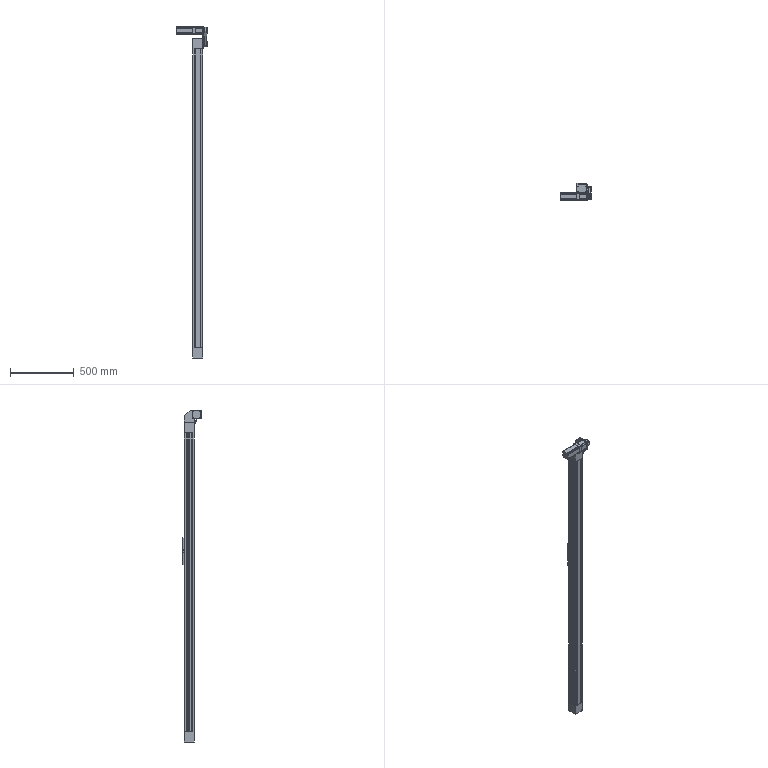Part | SolidWorks | 14 solids | 807 faces | box 249.5 x 142 x 2600 mm | volume 14332524 mm3 | plane 383 | cylinder 332 | cone 80 | torus 12 | commonest cylinder face diameters 38.65 x52 5 x39 5.5 x28 4 x26 3.3 x24 4.2 x18